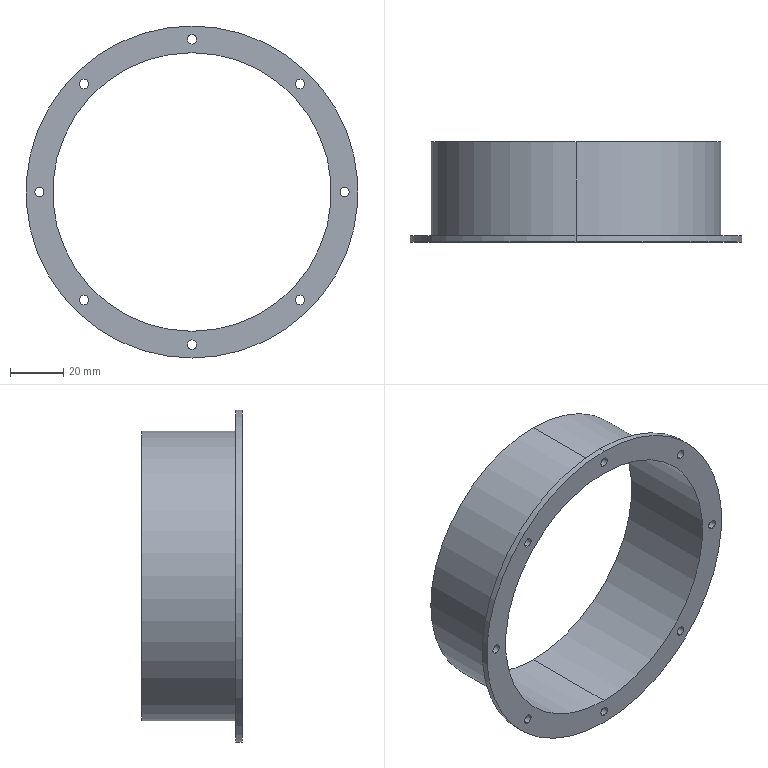Part | SolidWorks | features SavedExtBody 1 | 1 solid | 25 faces | box 124.775 x 37.645 x 124.775 mm | volume 33353 mm3 | cylinder 22 | plane 3 | commonest cylinder face diameters 3.5 x16 104.686 x2 108.906 x2 124.775 x2
STEP:
#1=CARTESIAN_POINT('',(-57.365,-225.737,66.75));
#2=VERTEX_POINT('',#1);
#3=CARTESIAN_POINT('',(-57.365,-225.737,63.25));
#4=VERTEX_POINT('',#3);
#5=CARTESIAN_POINT('',(-57.365,-225.737,65.));
#6=DIRECTION('',(0.,-1.,0.));
#7=DIRECTION('',(0.,0.,-1.));
#8=AXIS2_PLACEMENT_3D('',#5,#6,#7);
#9=CIRCLE('',#8,1.75);
#10=EDGE_CURVE('',#2,#4,#9,.T.);
#11=ORIENTED_EDGE('',*,*,#10,.F.);
#12=CARTESIAN_POINT('',(-57.365,-228.101,66.75));
#13=VERTEX_POINT('',#12);
#14=CARTESIAN_POINT('',(-57.365,-221.101,66.75));
#15=DIRECTION('',(0.,-1.,0.));
#16=VECTOR('',#15,1000.);
#17=LINE('',#14,#16);
#18=EDGE_CURVE('',#2,#13,#17,.T.);
#19=ORIENTED_EDGE('',*,*,#18,.T.);
#20=CARTESIAN_POINT('',(-57.365,-228.101,63.25));
#21=VERTEX_POINT('',#20);
#22=CARTESIAN_POINT('',(-57.365,-228.101,65.));
#23=DIRECTION('',(0.,-1.,0.));
#24=DIRECTION('',(0.,0.,-1.));
#25=AXIS2_PLACEMENT_3D('',#22,#23,#24);
#26=CIRCLE('',#25,1.75);
#27=EDGE_CURVE('',#13,#21,#26,.T.);
#28=ORIENTED_EDGE('',*,*,#27,.T.);
#29=CARTESIAN_POINT('',(-57.365,-221.101,63.25));
#30=DIRECTION('',(0.,-1.,0.));
#31=VECTOR('',#30,1000.);
#32=LINE('',#29,#31);
#33=EDGE_CURVE('',#4,#21,#32,.T.);
#34=ORIENTED_EDGE('',*,*,#33,.F.);
#35=EDGE_LOOP('',(#11,#19,#28,#34));
#36=FACE_OUTER_BOUND('',#35,.T.);
#37=CARTESIAN_POINT('',(-57.365,-221.101,65.));
#38=DIRECTION('',(0.,-1.,0.));
#39=DIRECTION('',(0.,0.,-1.));
#40=AXIS2_PLACEMENT_3D('',#37,#38,#39);
#41=CYLINDRICAL_SURFACE('',#40,1.75);
#42=ADVANCED_FACE('',(#36),#41,.F.);
#43=CARTESIAN_POINT('',(-40.563,-225.737,107.313));
#44=VERTEX_POINT('',#43);
#45=CARTESIAN_POINT('',(-40.563,-225.737,103.813));
#46=VERTEX_POINT('',#45);
#47=CARTESIAN_POINT('',(-40.563,-225.737,105.563));
#48=DIRECTION('',(0.,-1.,0.));
#49=DIRECTION('',(0.,0.,-1.));
#50=AXIS2_PLACEMENT_3D('',#47,#48,#49);
#51=CIRCLE('',#50,1.75);
#52=EDGE_CURVE('',#44,#46,#51,.T.);
#53=ORIENTED_EDGE('',*,*,#52,.F.);
#54=CARTESIAN_POINT('',(-40.563,-228.101,107.313));
#55=VERTEX_POINT('',#54);
#56=CARTESIAN_POINT('',(-40.563,-221.101,107.313));
#57=DIRECTION('',(0.,-1.,0.));
#58=VECTOR('',#57,1000.);
#59=LINE('',#56,#58);
#60=EDGE_CURVE('',#44,#55,#59,.T.);
#61=ORIENTED_EDGE('',*,*,#60,.T.);
#62=CARTESIAN_POINT('',(-40.563,-228.101,103.813));
#63=VERTEX_POINT('',#62);
#64=CARTESIAN_POINT('',(-40.563,-228.101,105.563));
#65=DIRECTION('',(0.,-1.,0.));
#66=DIRECTION('',(0.,0.,-1.));
#67=AXIS2_PLACEMENT_3D('',#64,#65,#66);
#68=CIRCLE('',#67,1.75);
#69=EDGE_CURVE('',#55,#63,#68,.T.);
#70=ORIENTED_EDGE('',*,*,#69,.T.);
#71=CARTESIAN_POINT('',(-40.563,-221.101,103.813));
#72=DIRECTION('',(0.,-1.,0.));
#73=VECTOR('',#72,1000.);
#74=LINE('',#71,#73);
#75=EDGE_CURVE('',#46,#63,#74,.T.);
#76=ORIENTED_EDGE('',*,*,#75,.F.);
#77=EDGE_LOOP('',(#53,#61,#70,#76));
#78=FACE_OUTER_BOUND('',#77,.T.);
#79=CARTESIAN_POINT('',(-40.563,-221.101,105.563));
#80=DIRECTION('',(0.,-1.,0.));
#81=DIRECTION('',(0.,0.,-1.));
#82=AXIS2_PLACEMENT_3D('',#79,#80,#81);
#83=CYLINDRICAL_SURFACE('',#82,1.75);
#84=ADVANCED_FACE('',(#78),#83,.F.);
#85=CARTESIAN_POINT('',(0.,-225.737,124.115));
#86=VERTEX_POINT('',#85);
#87=CARTESIAN_POINT('',(0.,-225.737,120.615));
#88=VERTEX_POINT('',#87);
#89=CARTESIAN_POINT('',(0.,-225.737,122.365));
#90=DIRECTION('',(0.,-1.,0.));
#91=DIRECTION('',(0.,0.,-1.));
#92=AXIS2_PLACEMENT_3D('',#89,#90,#91);
#93=CIRCLE('',#92,1.75);
#94=EDGE_CURVE('',#86,#88,#93,.T.);
#95=ORIENTED_EDGE('',*,*,#94,.F.);
#96=CARTESIAN_POINT('',(0.,-228.101,124.115));
#97=VERTEX_POINT('',#96);
#98=CARTESIAN_POINT('',(0.,-221.101,124.115));
#99=DIRECTION('',(0.,-1.,0.));
#100=VECTOR('',#99,1000.);
#101=LINE('',#98,#100);
#102=EDGE_CURVE('',#86,#97,#101,.T.);
#103=ORIENTED_EDGE('',*,*,#102,.T.);
#104=CARTESIAN_POINT('',(0.,-228.101,120.615));
#105=VERTEX_POINT('',#104);
#106=CARTESIAN_POINT('',(0.,-228.101,122.365));
#107=DIRECTION('',(0.,-1.,0.));
#108=DIRECTION('',(0.,0.,-1.));
#109=AXIS2_PLACEMENT_3D('',#106,#107,#108);
#110=CIRCLE('',#109,1.75);
#111=EDGE_CURVE('',#97,#105,#110,.T.);
#112=ORIENTED_EDGE('',*,*,#111,.T.);
#113=CARTESIAN_POINT('',(0.,-221.101,120.615));
#114=DIRECTION('',(0.,-1.,0.));
#115=VECTOR('',#114,1000.);
#116=LINE('',#113,#115);
#117=EDGE_CURVE('',#88,#105,#116,.T.);
#118=ORIENTED_EDGE('',*,*,#117,.F.);
#119=EDGE_LOOP('',(#95,#103,#112,#118));
#120=FACE_OUTER_BOUND('',#119,.T.);
#121=CARTESIAN_POINT('',(0.,-221.101,122.365));
#122=DIRECTION('',(0.,-1.,0.));
#123=DIRECTION('',(0.,0.,-1.));
#124=AXIS2_PLACEMENT_3D('',#121,#122,#123);
#125=CYLINDRICAL_SURFACE('',#124,1.75);
#126=ADVANCED_FACE('',(#120),#125,.F.);
#127=CARTESIAN_POINT('',(40.563,-225.737,107.313));
#128=VERTEX_POINT('',#127);
#129=CARTESIAN_POINT('',(40.563,-225.737,103.813));
#130=VERTEX_POINT('',#129);
#131=CARTESIAN_POINT('',(40.563,-225.737,105.563));
#132=DIRECTION('',(0.,-1.,0.));
#133=DIRECTION('',(0.,0.,-1.));
#134=AXIS2_PLACEMENT_3D('',#131,#132,#133);
#135=CIRCLE('',#134,1.75);
#136=EDGE_CURVE('',#128,#130,#135,.T.);
#137=ORIENTED_EDGE('',*,*,#136,.F.);
#138=CARTESIAN_POINT('',(40.563,-228.101,107.313));
#139=VERTEX_POINT('',#138);
#140=CARTESIAN_POINT('',(40.563,-221.101,107.313));
#141=DIRECTION('',(0.,-1.,0.));
#142=VECTOR('',#141,1000.);
#143=LINE('',#140,#142);
#144=EDGE_CURVE('',#128,#139,#143,.T.);
#145=ORIENTED_EDGE('',*,*,#144,.T.);
#146=CARTESIAN_POINT('',(40.563,-228.101,103.813));
#147=VERTEX_POINT('',#146);
#148=CARTESIAN_POINT('',(40.563,-228.101,105.563));
#149=DIRECTION('',(0.,-1.,0.));
#150=DIRECTION('',(0.,0.,-1.));
#151=AXIS2_PLACEMENT_3D('',#148,#149,#150);
#152=CIRCLE('',#151,1.75);
#153=EDGE_CURVE('',#139,#147,#152,.T.);
#154=ORIENTED_EDGE('',*,*,#153,.T.);
#155=CARTESIAN_POINT('',(40.563,-221.101,103.813));
#156=DIRECTION('',(0.,-1.,0.));
#157=VECTOR('',#156,1000.);
#158=LINE('',#155,#157);
#159=EDGE_CURVE('',#130,#147,#158,.T.);
#160=ORIENTED_EDGE('',*,*,#159,.F.);
#161=EDGE_LOOP('',(#137,#145,#154,#160));
#162=FACE_OUTER_BOUND('',#161,.T.);
#163=CARTESIAN_POINT('',(40.563,-221.101,105.563));
#164=DIRECTION('',(0.,-1.,0.));
#165=DIRECTION('',(0.,0.,-1.));
#166=AXIS2_PLACEMENT_3D('',#163,#164,#165);
#167=CYLINDRICAL_SURFACE('',#166,1.75);
#168=ADVANCED_FACE('',(#162),#167,.F.);
#169=CARTESIAN_POINT('',(57.365,-225.737,66.75));
#170=VERTEX_POINT('',#169);
#171=CARTESIAN_POINT('',(57.365,-225.737,63.25));
#172=VERTEX_POINT('',#171);
#173=CARTESIAN_POINT('',(57.365,-225.737,65.));
#174=DIRECTION('',(0.,-1.,0.));
#175=DIRECTION('',(0.,0.,-1.));
#176=AXIS2_PLACEMENT_3D('',#173,#174,#175);
#177=CIRCLE('',#176,1.75);
#178=EDGE_CURVE('',#170,#172,#177,.T.);
#179=ORIENTED_EDGE('',*,*,#178,.F.);
#180=CARTESIAN_POINT('',(57.365,-228.101,66.75));
#181=VERTEX_POINT('',#180);
#182=CARTESIAN_POINT('',(57.365,-221.101,66.75));
#183=DIRECTION('',(0.,-1.,0.));
#184=VECTOR('',#183,1000.);
#185=LINE('',#182,#184);
#186=EDGE_CURVE('',#170,#181,#185,.T.);
#187=ORIENTED_EDGE('',*,*,#186,.T.);
#188=CARTESIAN_POINT('',(57.365,-228.101,63.25));
#189=VERTEX_POINT('',#188);
#190=CARTESIAN_POINT('',(57.365,-228.101,65.));
#191=DIRECTION('',(0.,-1.,0.));
#192=DIRECTION('',(0.,0.,-1.));
#193=AXIS2_PLACEMENT_3D('',#190,#191,#192);
#194=CIRCLE('',#193,1.75);
#195=EDGE_CURVE('',#181,#189,#194,.T.);
#196=ORIENTED_EDGE('',*,*,#195,.T.);
#197=CARTESIAN_POINT('',(57.365,-221.101,63.25));
#198=DIRECTION('',(0.,-1.,0.));
#199=VECTOR('',#198,1000.);
#200=LINE('',#197,#199);
#201=EDGE_CURVE('',#172,#189,#200,.T.);
#202=ORIENTED_EDGE('',*,*,#201,.F.);
#203=EDGE_LOOP('',(#179,#187,#196,#202));
#204=FACE_OUTER_BOUND('',#203,.T.);
#205=CARTESIAN_POINT('',(57.365,-221.101,65.));
#206=DIRECTION('',(0.,-1.,0.));
#207=DIRECTION('',(0.,0.,-1.));
#208=AXIS2_PLACEMENT_3D('',#205,#206,#207);
#209=CYLINDRICAL_SURFACE('',#208,1.75);
#210=ADVANCED_FACE('',(#204),#209,.F.);
#211=CARTESIAN_POINT('',(40.563,-225.737,26.187));
#212=VERTEX_POINT('',#211);
#213=CARTESIAN_POINT('',(40.563,-225.737,22.687));
#214=VERTEX_POINT('',#213);
#215=CARTESIAN_POINT('',(40.563,-225.737,24.437));
#216=DIRECTION('',(0.,-1.,0.));
#217=DIRECTION('',(0.,0.,-1.));
#218=AXIS2_PLACEMENT_3D('',#215,#216,#217);
#219=CIRCLE('',#218,1.75);
#220=EDGE_CURVE('',#212,#214,#219,.T.);
#221=ORIENTED_EDGE('',*,*,#220,.F.);
#222=CARTESIAN_POINT('',(40.563,-228.101,26.187));
#223=VERTEX_POINT('',#222);
#224=CARTESIAN_POINT('',(40.563,-221.101,26.187));
#225=DIRECTION('',(0.,-1.,0.));
#226=VECTOR('',#225,1000.);
#227=LINE('',#224,#226);
#228=EDGE_CURVE('',#212,#223,#227,.T.);
#229=ORIENTED_EDGE('',*,*,#228,.T.);
#230=CARTESIAN_POINT('',(40.563,-228.101,22.687));
#231=VERTEX_POINT('',#230);
#232=CARTESIAN_POINT('',(40.563,-228.101,24.437));
#233=DIRECTION('',(0.,-1.,0.));
#234=DIRECTION('',(0.,0.,-1.));
#235=AXIS2_PLACEMENT_3D('',#232,#233,#234);
#236=CIRCLE('',#235,1.75);
#237=EDGE_CURVE('',#223,#231,#236,.T.);
#238=ORIENTED_EDGE('',*,*,#237,.T.);
#239=CARTESIAN_POINT('',(40.563,-221.101,22.687));
#240=DIRECTION('',(0.,-1.,0.));
#241=VECTOR('',#240,1000.);
#242=LINE('',#239,#241);
#243=EDGE_CURVE('',#214,#231,#242,.T.);
#244=ORIENTED_EDGE('',*,*,#243,.F.);
#245=EDGE_LOOP('',(#221,#229,#238,#244));
#246=FACE_OUTER_BOUND('',#245,.T.);
#247=CARTESIAN_POINT('',(40.563,-221.101,24.437));
#248=DIRECTION('',(0.,-1.,0.));
#249=DIRECTION('',(0.,0.,-1.));
#250=AXIS2_PLACEMENT_3D('',#247,#248,#249);
#251=CYLINDRICAL_SURFACE('',#250,1.75);
#252=ADVANCED_FACE('',(#246),#251,.F.);
#253=CARTESIAN_POINT('',(0.,-225.737,9.385));
#254=VERTEX_POINT('',#253);
#255=CARTESIAN_POINT('',(0.,-225.737,5.885));
#256=VERTEX_POINT('',#255);
#257=CARTESIAN_POINT('',(0.,-225.737,7.635));
#258=DIRECTION('',(0.,-1.,0.));
#259=DIRECTION('',(0.,0.,-1.));
#260=AXIS2_PLACEMENT_3D('',#257,#258,#259);
#261=CIRCLE('',#260,1.75);
#262=EDGE_CURVE('',#254,#256,#261,.T.);
#263=ORIENTED_EDGE('',*,*,#262,.F.);
#264=CARTESIAN_POINT('',(0.,-228.101,9.385));
#265=VERTEX_POINT('',#264);
#266=CARTESIAN_POINT('',(0.,-221.101,9.385));
#267=DIRECTION('',(0.,-1.,0.));
#268=VECTOR('',#267,1000.);
#269=LINE('',#266,#268);
#270=EDGE_CURVE('',#254,#265,#269,.T.);
#271=ORIENTED_EDGE('',*,*,#270,.T.);
#272=CARTESIAN_POINT('',(0.,-228.101,5.885));
#273=VERTEX_POINT('',#272);
#274=CARTESIAN_POINT('',(0.,-228.101,7.635));
#275=DIRECTION('',(0.,-1.,0.));
#276=DIRECTION('',(0.,0.,-1.));
#277=AXIS2_PLACEMENT_3D('',#274,#275,#276);
#278=CIRCLE('',#277,1.75);
#279=EDGE_CURVE('',#265,#273,#278,.T.);
#280=ORIENTED_EDGE('',*,*,#279,.T.);
#281=CARTESIAN_POINT('',(0.,-221.101,5.885));
#282=DIRECTION('',(0.,-1.,0.));
#283=VECTOR('',#282,1000.);
#284=LINE('',#281,#283);
#285=EDGE_CURVE('',#256,#273,#284,.T.);
#286=ORIENTED_EDGE('',*,*,#285,.F.);
#287=EDGE_LOOP('',(#263,#271,#280,#286));
#288=FACE_OUTER_BOUND('',#287,.T.);
#289=CARTESIAN_POINT('',(0.,-221.101,7.635));
#290=DIRECTION('',(0.,-1.,0.));
#291=DIRECTION('',(0.,0.,-1.));
#292=AXIS2_PLACEMENT_3D('',#289,#290,#291);
#293=CYLINDRICAL_SURFACE('',#292,1.75);
#294=ADVANCED_FACE('',(#288),#293,.F.);
#295=CARTESIAN_POINT('',(-40.563,-225.737,26.187));
#296=VERTEX_POINT('',#295);
#297=CARTESIAN_POINT('',(-40.563,-225.737,22.687));
#298=VERTEX_POINT('',#297);
#299=CARTESIAN_POINT('',(-40.563,-225.737,24.437));
#300=DIRECTION('',(0.,-1.,0.));
#301=DIRECTION('',(0.,0.,-1.));
#302=AXIS2_PLACEMENT_3D('',#299,#300,#301);
#303=CIRCLE('',#302,1.75);
#304=EDGE_CURVE('',#296,#298,#303,.T.);
#305=ORIENTED_EDGE('',*,*,#304,.F.);
#306=CARTESIAN_POINT('',(-40.563,-228.101,26.187));
#307=VERTEX_POINT('',#306);
#308=CARTESIAN_POINT('',(-40.563,-221.101,26.187));
#309=DIRECTION('',(0.,-1.,0.));
#310=VECTOR('',#309,1000.);
#311=LINE('',#308,#310);
#312=EDGE_CURVE('',#296,#307,#311,.T.);
#313=ORIENTED_EDGE('',*,*,#312,.T.);
#314=CARTESIAN_POINT('',(-40.563,-228.101,22.687));
#315=VERTEX_POINT('',#314);
#316=CARTESIAN_POINT('',(-40.563,-228.101,24.437));
#317=DIRECTION('',(0.,-1.,0.));
#318=DIRECTION('',(0.,0.,-1.));
#319=AXIS2_PLACEMENT_3D('',#316,#317,#318);
#320=CIRCLE('',#319,1.75);
#321=EDGE_CURVE('',#307,#315,#320,.T.);
#322=ORIENTED_EDGE('',*,*,#321,.T.);
#323=CARTESIAN_POINT('',(-40.563,-221.101,22.687));
#324=DIRECTION('',(0.,-1.,0.));
#325=VECTOR('',#324,1000.);
#326=LINE('',#323,#325);
#327=EDGE_CURVE('',#298,#315,#326,.T.);
#328=ORIENTED_EDGE('',*,*,#327,.F.);
#329=EDGE_LOOP('',(#305,#313,#322,#328));
#330=FACE_OUTER_BOUND('',#329,.T.);
#331=CARTESIAN_POINT('',(-40.563,-221.101,24.437));
#332=DIRECTION('',(0.,-1.,0.));
#333=DIRECTION('',(0.,0.,-1.));
#334=AXIS2_PLACEMENT_3D('',#331,#332,#333);
#335=CYLINDRICAL_SURFACE('',#334,1.75);
#336=ADVANCED_FACE('',(#330),#335,.F.);
#337=CARTESIAN_POINT('',(0.,-190.456,10.547));
#338=VERTEX_POINT('',#337);
#339=CARTESIAN_POINT('',(0.,-190.456,119.453));
#340=VERTEX_POINT('',#339);
#341=CARTESIAN_POINT('',(0.,-190.456,65.));
#342=DIRECTION('',(0.,-1.,0.));
#343=DIRECTION('',(0.,0.,-1.));
#344=AXIS2_PLACEMENT_3D('',#341,#342,#343);
#345=CIRCLE('',#344,54.453);
#346=EDGE_CURVE('',#338,#340,#345,.T.);
#347=ORIENTED_EDGE('',*,*,#346,.T.);
#348=CARTESIAN_POINT('',(0.,-225.737,119.453));
#349=VERTEX_POINT('',#348);
#350=CARTESIAN_POINT('',(0.,-253.035,119.453));
#351=DIRECTION('',(0.,-1.,0.));
#352=VECTOR('',#351,1000.);
#353=LINE('',#350,#352);
#354=EDGE_CURVE('',#340,#349,#353,.T.);
#355=ORIENTED_EDGE('',*,*,#354,.T.);
#356=CARTESIAN_POINT('',(0.,-225.737,10.547));
#357=VERTEX_POINT('',#356);
#358=CARTESIAN_POINT('',(0.,-225.737,65.));
#359=DIRECTION('',(0.,-1.,0.));
#360=DIRECTION('',(0.,0.,-1.));
#361=AXIS2_PLACEMENT_3D('',#358,#359,#360);
#362=CIRCLE('',#361,54.453);
#363=EDGE_CURVE('',#357,#349,#362,.T.);
#364=ORIENTED_EDGE('',*,*,#363,.F.);
#365=CARTESIAN_POINT('',(0.,-253.035,10.547));
#366=DIRECTION('',(0.,-1.,0.));
#367=VECTOR('',#366,1000.);
#368=LINE('',#365,#367);
#369=EDGE_CURVE('',#338,#357,#368,.T.);
#370=ORIENTED_EDGE('',*,*,#369,.F.);
#371=EDGE_LOOP('',(#347,#355,#364,#370));
#372=FACE_OUTER_BOUND('',#371,.T.);
#373=CARTESIAN_POINT('',(0.,-253.035,65.));
#374=DIRECTION('',(0.,-1.,0.));
#375=DIRECTION('',(0.,0.,-1.));
#376=AXIS2_PLACEMENT_3D('',#373,#374,#375);
#377=CYLINDRICAL_SURFACE('',#376,54.453);
#378=ADVANCED_FACE('',(#372),#377,.T.);
#379=CARTESIAN_POINT('',(0.,-225.737,2.613));
#380=VERTEX_POINT('',#379);
#381=CARTESIAN_POINT('',(0.,-225.737,127.387));
#382=VERTEX_POINT('',#381);
#383=CARTESIAN_POINT('',(0.,-225.737,65.));
#384=DIRECTION('',(0.,-1.,0.));
#385=DIRECTION('',(0.,0.,-1.));
#386=AXIS2_PLACEMENT_3D('',#383,#384,#385);
#387=CIRCLE('',#386,62.387);
#388=EDGE_CURVE('',#380,#382,#387,.T.);
#389=ORIENTED_EDGE('',*,*,#388,.T.);
#390=CARTESIAN_POINT('',(0.,-228.101,127.387));
#391=VERTEX_POINT('',#390);
#392=CARTESIAN_POINT('',(0.,-253.035,127.387));
#393=DIRECTION('',(0.,-1.,0.));
#394=VECTOR('',#393,1000.);
#395=LINE('',#392,#394);
#396=EDGE_CURVE('',#382,#391,#395,.T.);
#397=ORIENTED_EDGE('',*,*,#396,.T.);
#398=CARTESIAN_POINT('',(0.,-228.101,2.613));
#399=VERTEX_POINT('',#398);
#400=CARTESIAN_POINT('',(0.,-228.101,65.));
#401=DIRECTION('',(0.,-1.,0.));
#402=DIRECTION('',(0.,0.,-1.));
#403=AXIS2_PLACEMENT_3D('',#400,#401,#402);
#404=CIRCLE('',#403,62.387);
#405=EDGE_CURVE('',#399,#391,#404,.T.);
#406=ORIENTED_EDGE('',*,*,#405,.F.);
#407=CARTESIAN_POINT('',(0.,-253.035,2.613));
#408=DIRECTION('',(0.,-1.,0.));
#409=VECTOR('',#408,1000.);
#410=LINE('',#407,#409);
#411=EDGE_CURVE('',#380,#399,#410,.T.);
#412=ORIENTED_EDGE('',*,*,#411,.F.);
#413=EDGE_LOOP('',(#389,#397,#406,#412));
#414=FACE_OUTER_BOUND('',#413,.T.);
#415=CARTESIAN_POINT('',(0.,-253.035,65.));
#416=DIRECTION('',(0.,-1.,0.));
#417=DIRECTION('',(0.,0.,-1.));
#418=AXIS2_PLACEMENT_3D('',#415,#416,#417);
#419=CYLINDRICAL_SURFACE('',#418,62.387);
#420=ADVANCED_FACE('',(#414),#419,.T.);
#421=CARTESIAN_POINT('',(0.,-190.456,117.343));
#422=VERTEX_POINT('',#421);
#423=CARTESIAN_POINT('',(0.,-190.456,12.657));
#424=VERTEX_POINT('',#423);
#425=CARTESIAN_POINT('',(0.,-190.456,65.));
#426=DIRECTION('',(0.,-1.,0.));
#427=DIRECTION('',(0.,0.,-1.));
#428=AXIS2_PLACEMENT_3D('',#425,#426,#427);
#429=CIRCLE('',#428,52.343);
#430=EDGE_CURVE('',#422,#424,#429,.T.);
#431=ORIENTED_EDGE('',*,*,#430,.F.);
#432=CARTESIAN_POINT('',(0.,-228.101,117.343));
#433=VERTEX_POINT('',#432);
#434=CARTESIAN_POINT('',(0.,-253.035,117.343));
#435=DIRECTION('',(0.,-1.,0.));
#436=VECTOR('',#435,1000.);
#437=LINE('',#434,#436);
#438=EDGE_CURVE('',#422,#433,#437,.T.);
#439=ORIENTED_EDGE('',*,*,#438,.T.);
#440=CARTESIAN_POINT('',(0.,-228.101,12.657));
#441=VERTEX_POINT('',#440);
#442=CARTESIAN_POINT('',(0.,-228.101,65.));
#443=DIRECTION('',(0.,-1.,0.));
#444=DIRECTION('',(0.,0.,-1.));
#445=AXIS2_PLACEMENT_3D('',#442,#443,#444);
#446=CIRCLE('',#445,52.343);
#447=EDGE_CURVE('',#433,#441,#446,.T.);
#448=ORIENTED_EDGE('',*,*,#447,.T.);
#449=CARTESIAN_POINT('',(0.,-253.035,12.657));
#450=DIRECTION('',(0.,-1.,0.));
#451=VECTOR('',#450,1000.);
#452=LINE('',#449,#451);
#453=EDGE_CURVE('',#424,#441,#452,.T.);
#454=ORIENTED_EDGE('',*,*,#453,.F.);
#455=EDGE_LOOP('',(#431,#439,#448,#454));
#456=FACE_OUTER_BOUND('',#455,.T.);
#457=CARTESIAN_POINT('',(0.,-253.035,65.));
#458=DIRECTION('',(0.,-1.,0.));
#459=DIRECTION('',(0.,0.,-1.));
#460=AXIS2_PLACEMENT_3D('',#457,#458,#459);
#461=CYLINDRICAL_SURFACE('',#460,52.343);
#462=ADVANCED_FACE('',(#456),#461,.F.);
#463=ORIENTED_EDGE('',*,*,#438,.F.);
#464=CARTESIAN_POINT('',(0.,-190.456,65.));
#465=DIRECTION('',(0.,-1.,0.));
#466=DIRECTION('',(0.,0.,-1.));
#467=AXIS2_PLACEMENT_3D('',#464,#465,#466);
#468=CIRCLE('',#467,52.343);
#469=EDGE_CURVE('',#424,#422,#468,.T.);
#470=ORIENTED_EDGE('',*,*,#469,.F.);
#471=ORIENTED_EDGE('',*,*,#453,.T.);
#472=CARTESIAN_POINT('',(0.,-228.101,65.));
#473=DIRECTION('',(0.,-1.,0.));
#474=DIRECTION('',(0.,0.,-1.));
#475=AXIS2_PLACEMENT_3D('',#472,#473,#474);
#476=CIRCLE('',#475,52.343);
#477=EDGE_CURVE('',#441,#433,#476,.T.);
#478=ORIENTED_EDGE('',*,*,#477,.T.);
#479=EDGE_LOOP('',(#463,#470,#471,#478));
#480=FACE_OUTER_BOUND('',#479,.T.);
#481=CARTESIAN_POINT('',(0.,-253.035,65.));
#482=DIRECTION('',(0.,-1.,0.));
#483=DIRECTION('',(0.,0.,-1.));
#484=AXIS2_PLACEMENT_3D('',#481,#482,#483);
#485=CYLINDRICAL_SURFACE('',#484,52.343);
#486=ADVANCED_FACE('',(#480),#485,.F.);
#487=CARTESIAN_POINT('',(-57.365,-228.101,65.));
#488=DIRECTION('',(0.,-1.,0.));
#489=DIRECTION('',(0.,0.,-1.));
#490=AXIS2_PLACEMENT_3D('',#487,#488,#489);
#491=CIRCLE('',#490,1.75);
#492=EDGE_CURVE('',#21,#13,#491,.T.);
#493=ORIENTED_EDGE('',*,*,#492,.F.);
#494=ORIENTED_EDGE('',*,*,#27,.F.);
#495=EDGE_LOOP('',(#493,#494));
#496=FACE_BOUND('',#495,.T.);
#497=CARTESIAN_POINT('',(-40.563,-228.101,105.563));
#498=DIRECTION('',(0.,-1.,0.));
#499=DIRECTION('',(0.,0.,-1.));
#500=AXIS2_PLACEMENT_3D('',#497,#498,#499);
#501=CIRCLE('',#500,1.75);
#502=EDGE_CURVE('',#63,#55,#501,.T.);
#503=ORIENTED_EDGE('',*,*,#502,.F.);
#504=ORIENTED_EDGE('',*,*,#69,.F.);
#505=EDGE_LOOP('',(#503,#504));
#506=FACE_BOUND('',#505,.T.);
#507=CARTESIAN_POINT('',(0.,-228.101,122.365));
#508=DIRECTION('',(0.,-1.,0.));
#509=DIRECTION('',(0.,0.,-1.));
#510=AXIS2_PLACEMENT_3D('',#507,#508,#509);
#511=CIRCLE('',#510,1.75);
#512=EDGE_CURVE('',#105,#97,#511,.T.);
#513=ORIENTED_EDGE('',*,*,#512,.F.);
#514=ORIENTED_EDGE('',*,*,#111,.F.);
#515=EDGE_LOOP('',(#513,#514));
#516=FACE_BOUND('',#515,.T.);
#517=CARTESIAN_POINT('',(40.563,-228.101,105.563));
#518=DIRECTION('',(0.,-1.,0.));
#519=DIRECTION('',(0.,0.,-1.));
#520=AXIS2_PLACEMENT_3D('',#517,#518,#519);
#521=CIRCLE('',#520,1.75);
#522=EDGE_CURVE('',#147,#139,#521,.T.);
#523=ORIENTED_EDGE('',*,*,#522,.F.);
#524=ORIENTED_EDGE('',*,*,#153,.F.);
#525=EDGE_LOOP('',(#523,#524));
#526=FACE_BOUND('',#525,.T.);
#527=CARTESIAN_POINT('',(57.365,-228.101,65.));
#528=DIRECTION('',(0.,-1.,0.));
#529=DIRECTION('',(0.,0.,-1.));
#530=AXIS2_PLACEMENT_3D('',#527,#528,#529);
#531=CIRCLE('',#530,1.75);
#532=EDGE_CURVE('',#189,#181,#531,.T.);
#533=ORIENTED_EDGE('',*,*,#532,.F.);
#534=ORIENTED_EDGE('',*,*,#195,.F.);
#535=EDGE_LOOP('',(#533,#534));
#536=FACE_BOUND('',#535,.T.);
#537=CARTESIAN_POINT('',(40.563,-228.101,24.437));
#538=DIRECTION('',(0.,-1.,0.));
#539=DIRECTION('',(0.,0.,-1.));
#540=AXIS2_PLACEMENT_3D('',#537,#538,#539);
#541=CIRCLE('',#540,1.75);
#542=EDGE_CURVE('',#231,#223,#541,.T.);
#543=ORIENTED_EDGE('',*,*,#542,.F.);
#544=ORIENTED_EDGE('',*,*,#237,.F.);
#545=EDGE_LOOP('',(#543,#544));
#546=FACE_BOUND('',#545,.T.);
#547=CARTESIAN_POINT('',(0.,-228.101,7.635));
#548=DIRECTION('',(0.,-1.,0.));
#549=DIRECTION('',(0.,0.,-1.));
#550=AXIS2_PLACEMENT_3D('',#547,#548,#549);
#551=CIRCLE('',#550,1.75);
#552=EDGE_CURVE('',#273,#265,#551,.T.);
#553=ORIENTED_EDGE('',*,*,#552,.F.);
#554=ORIENTED_EDGE('',*,*,#279,.F.);
#555=EDGE_LOOP('',(#553,#554));
#556=FACE_BOUND('',#555,.T.);
#557=CARTESIAN_POINT('',(-40.563,-228.101,24.437));
#558=DIRECTION('',(0.,-1.,0.));
#559=DIRECTION('',(0.,0.,-1.));
#560=AXIS2_PLACEMENT_3D('',#557,#558,#559);
#561=CIRCLE('',#560,1.75);
#562=EDGE_CURVE('',#315,#307,#561,.T.);
#563=ORIENTED_EDGE('',*,*,#562,.F.);
#564=ORIENTED_EDGE('',*,*,#321,.F.);
#565=EDGE_LOOP('',(#563,#564));
#566=FACE_BOUND('',#565,.T.);
#567=ORIENTED_EDGE('',*,*,#477,.F.);
#568=ORIENTED_EDGE('',*,*,#447,.F.);
#569=EDGE_LOOP('',(#567,#568));
#570=FACE_BOUND('',#569,.T.);
#571=ORIENTED_EDGE('',*,*,#405,.T.);
#572=CARTESIAN_POINT('',(0.,-228.101,65.));
#573=DIRECTION('',(0.,-1.,0.));
#574=DIRECTION('',(0.,0.,-1.));
#575=AXIS2_PLACEMENT_3D('',#572,#573,#574);
#576=CIRCLE('',#575,62.387);
#577=EDGE_CURVE('',#391,#399,#576,.T.);
#578=ORIENTED_EDGE('',*,*,#577,.T.);
#579=EDGE_LOOP('',(#571,#578));
#580=FACE_OUTER_BOUND('',#579,.T.);
#581=CARTESIAN_POINT('',(-54.453,-228.101,65.));
#582=DIRECTION('',(0.,1.,0.));
#583=DIRECTION('',(0.,0.,1.));
#584=AXIS2_PLACEMENT_3D('',#581,#582,#583);
#585=PLANE('',#584);
#586=ADVANCED_FACE('',(#496,#506,#516,#526,#536,#546,#556,#566,#570,#580),#585,.F.);
#587=ORIENTED_EDGE('',*,*,#396,.F.);
#588=CARTESIAN_POINT('',(0.,-225.737,65.));
#589=DIRECTION('',(0.,-1.,0.));
#590=DIRECTION('',(0.,0.,-1.));
#591=AXIS2_PLACEMENT_3D('',#588,#589,#590);
#592=CIRCLE('',#591,62.387);
#593=EDGE_CURVE('',#382,#380,#592,.T.);
#594=ORIENTED_EDGE('',*,*,#593,.T.);
#595=ORIENTED_EDGE('',*,*,#411,.T.);
#596=ORIENTED_EDGE('',*,*,#577,.F.);
#597=EDGE_LOOP('',(#587,#594,#595,#596));
#598=FACE_OUTER_BOUND('',#597,.T.);
#599=CARTESIAN_POINT('',(0.,-253.035,65.));
#600=DIRECTION('',(0.,-1.,0.));
#601=DIRECTION('',(0.,0.,-1.));
#602=AXIS2_PLACEMENT_3D('',#599,#600,#601);
#603=CYLINDRICAL_SURFACE('',#602,62.387);
#604=ADVANCED_FACE('',(#598),#603,.T.);
#605=CARTESIAN_POINT('',(-57.365,-225.737,65.));
#606=DIRECTION('',(0.,-1.,0.));
#607=DIRECTION('',(0.,0.,-1.));
#608=AXIS2_PLACEMENT_3D('',#605,#606,#607);
#609=CIRCLE('',#608,1.75);
#610=EDGE_CURVE('',#4,#2,#609,.T.);
#611=ORIENTED_EDGE('',*,*,#610,.T.);
#612=ORIENTED_EDGE('',*,*,#10,.T.);
#613=EDGE_LOOP('',(#611,#612));
#614=FACE_BOUND('',#613,.T.);
#615=CARTESIAN_POINT('',(-40.563,-225.737,105.563));
#616=DIRECTION('',(0.,-1.,0.));
#617=DIRECTION('',(0.,0.,-1.));
#618=AXIS2_PLACEMENT_3D('',#615,#616,#617);
#619=CIRCLE('',#618,1.75);
#620=EDGE_CURVE('',#46,#44,#619,.T.);
#621=ORIENTED_EDGE('',*,*,#620,.T.);
#622=ORIENTED_EDGE('',*,*,#52,.T.);
#623=EDGE_LOOP('',(#621,#622));
#624=FACE_BOUND('',#623,.T.);
#625=CARTESIAN_POINT('',(0.,-225.737,122.365));
#626=DIRECTION('',(0.,-1.,0.));
#627=DIRECTION('',(0.,0.,-1.));
#628=AXIS2_PLACEMENT_3D('',#625,#626,#627);
#629=CIRCLE('',#628,1.75);
#630=EDGE_CURVE('',#88,#86,#629,.T.);
#631=ORIENTED_EDGE('',*,*,#630,.T.);
#632=ORIENTED_EDGE('',*,*,#94,.T.);
#633=EDGE_LOOP('',(#631,#632));
#634=FACE_BOUND('',#633,.T.);
#635=CARTESIAN_POINT('',(40.563,-225.737,105.563));
#636=DIRECTION('',(0.,-1.,0.));
#637=DIRECTION('',(0.,0.,-1.));
#638=AXIS2_PLACEMENT_3D('',#635,#636,#637);
#639=CIRCLE('',#638,1.75);
#640=EDGE_CURVE('',#130,#128,#639,.T.);
#641=ORIENTED_EDGE('',*,*,#640,.T.);
#642=ORIENTED_EDGE('',*,*,#136,.T.);
#643=EDGE_LOOP('',(#641,#642));
#644=FACE_BOUND('',#643,.T.);
#645=CARTESIAN_POINT('',(57.365,-225.737,65.));
#646=DIRECTION('',(0.,-1.,0.));
#647=DIRECTION('',(0.,0.,-1.));
#648=AXIS2_PLACEMENT_3D('',#645,#646,#647);
#649=CIRCLE('',#648,1.75);
#650=EDGE_CURVE('',#172,#170,#649,.T.);
#651=ORIENTED_EDGE('',*,*,#650,.T.);
#652=ORIENTED_EDGE('',*,*,#178,.T.);
#653=EDGE_LOOP('',(#651,#652));
#654=FACE_BOUND('',#653,.T.);
#655=CARTESIAN_POINT('',(40.563,-225.737,24.437));
#656=DIRECTION('',(0.,-1.,0.));
#657=DIRECTION('',(0.,0.,-1.));
#658=AXIS2_PLACEMENT_3D('',#655,#656,#657);
#659=CIRCLE('',#658,1.75);
#660=EDGE_CURVE('',#214,#212,#659,.T.);
#661=ORIENTED_EDGE('',*,*,#660,.T.);
#662=ORIENTED_EDGE('',*,*,#220,.T.);
#663=EDGE_LOOP('',(#661,#662));
#664=FACE_BOUND('',#663,.T.);
#665=CARTESIAN_POINT('',(0.,-225.737,7.635));
#666=DIRECTION('',(0.,-1.,0.));
#667=DIRECTION('',(0.,0.,-1.));
#668=AXIS2_PLACEMENT_3D('',#665,#666,#667);
#669=CIRCLE('',#668,1.75);
#670=EDGE_CURVE('',#256,#254,#669,.T.);
#671=ORIENTED_EDGE('',*,*,#670,.T.);
#672=ORIENTED_EDGE('',*,*,#262,.T.);
#673=EDGE_LOOP('',(#671,#672));
#674=FACE_BOUND('',#673,.T.);
#675=CARTESIAN_POINT('',(-40.563,-225.737,24.437));
#676=DIRECTION('',(0.,-1.,0.));
#677=DIRECTION('',(0.,0.,-1.));
#678=AXIS2_PLACEMENT_3D('',#675,#676,#677);
#679=CIRCLE('',#678,1.75);
#680=EDGE_CURVE('',#298,#296,#679,.T.);
#681=ORIENTED_EDGE('',*,*,#680,.T.);
#682=ORIENTED_EDGE('',*,*,#304,.T.);
#683=EDGE_LOOP('',(#681,#682));
#684=FACE_BOUND('',#683,.T.);
#685=ORIENTED_EDGE('',*,*,#388,.F.);
#686=ORIENTED_EDGE('',*,*,#593,.F.);
#687=EDGE_LOOP('',(#685,#686));
#688=FACE_OUTER_BOUND('',#687,.T.);
#689=ORIENTED_EDGE('',*,*,#363,.T.);
#690=CARTESIAN_POINT('',(0.,-225.737,65.));
#691=DIRECTION('',(0.,-1.,0.));
#692=DIRECTION('',(0.,0.,-1.));
#693=AXIS2_PLACEMENT_3D('',#690,#691,#692);
#694=CIRCLE('',#693,54.453);
#695=EDGE_CURVE('',#349,#357,#694,.T.);
#696=ORIENTED_EDGE('',*,*,#695,.T.);
#697=EDGE_LOOP('',(#689,#696));
#698=FACE_BOUND('',#697,.T.);
#699=CARTESIAN_POINT('',(-54.453,-225.737,65.));
#700=DIRECTION('',(0.,-1.,0.));
#701=DIRECTION('',(0.,0.,-1.));
#702=AXIS2_PLACEMENT_3D('',#699,#700,#701);
#703=PLANE('',#702);
#704=ADVANCED_FACE('',(#614,#624,#634,#644,#654,#664,#674,#684,#688,#698),#703,.F.);
#705=ORIENTED_EDGE('',*,*,#354,.F.);
#706=CARTESIAN_POINT('',(0.,-190.456,65.));
#707=DIRECTION('',(0.,-1.,0.));
#708=DIRECTION('',(0.,0.,-1.));
#709=AXIS2_PLACEMENT_3D('',#706,#707,#708);
#710=CIRCLE('',#709,54.453);
#711=EDGE_CURVE('',#340,#338,#710,.T.);
#712=ORIENTED_EDGE('',*,*,#711,.T.);
#713=ORIENTED_EDGE('',*,*,#369,.T.);
#714=ORIENTED_EDGE('',*,*,#695,.F.);
#715=EDGE_LOOP('',(#705,#712,#713,#714));
#716=FACE_OUTER_BOUND('',#715,.T.);
#717=CARTESIAN_POINT('',(0.,-253.035,65.));
#718=DIRECTION('',(0.,-1.,0.));
#719=DIRECTION('',(0.,0.,-1.));
#720=AXIS2_PLACEMENT_3D('',#717,#718,#719);
#721=CYLINDRICAL_SURFACE('',#720,54.453);
#722=ADVANCED_FACE('',(#716),#721,.T.);
#723=ORIENTED_EDGE('',*,*,#346,.F.);
#724=ORIENTED_EDGE('',*,*,#711,.F.);
#725=EDGE_LOOP('',(#723,#724));
#726=FACE_OUTER_BOUND('',#725,.T.);
#727=ORIENTED_EDGE('',*,*,#469,.T.);
#728=ORIENTED_EDGE('',*,*,#430,.T.);
#729=EDGE_LOOP('',(#727,#728));
#730=FACE_BOUND('',#729,.T.);
#731=CARTESIAN_POINT('',(-52.343,-190.456,65.));
#732=DIRECTION('',(0.,-1.,0.));
#733=DIRECTION('',(0.,0.,-1.));
#734=AXIS2_PLACEMENT_3D('',#731,#732,#733);
#735=PLANE('',#734);
#736=ADVANCED_FACE('',(#726,#730),#735,.F.);
#737=ORIENTED_EDGE('',*,*,#312,.F.);
#738=ORIENTED_EDGE('',*,*,#680,.F.);
#739=ORIENTED_EDGE('',*,*,#327,.T.);
#740=ORIENTED_EDGE('',*,*,#562,.T.);
#741=EDGE_LOOP('',(#737,#738,#739,#740));
#742=FACE_OUTER_BOUND('',#741,.T.);
#743=CARTESIAN_POINT('',(-40.563,-221.101,24.437));
#744=DIRECTION('',(0.,-1.,0.));
#745=DIRECTION('',(0.,0.,-1.));
#746=AXIS2_PLACEMENT_3D('',#743,#744,#745);
#747=CYLINDRICAL_SURFACE('',#746,1.75);
#748=ADVANCED_FACE('',(#742),#747,.F.);
#749=ORIENTED_EDGE('',*,*,#270,.F.);
#750=ORIENTED_EDGE('',*,*,#670,.F.);
#751=ORIENTED_EDGE('',*,*,#285,.T.);
#752=ORIENTED_EDGE('',*,*,#552,.T.);
#753=EDGE_LOOP('',(#749,#750,#751,#752));
#754=FACE_OUTER_BOUND('',#753,.T.);
#755=CARTESIAN_POINT('',(0.,-221.101,7.635));
#756=DIRECTION('',(0.,-1.,0.));
#757=DIRECTION('',(0.,0.,-1.));
#758=AXIS2_PLACEMENT_3D('',#755,#756,#757);
#759=CYLINDRICAL_SURFACE('',#758,1.75);
#760=ADVANCED_FACE('',(#754),#759,.F.);
#761=ORIENTED_EDGE('',*,*,#228,.F.);
#762=ORIENTED_EDGE('',*,*,#660,.F.);
#763=ORIENTED_EDGE('',*,*,#243,.T.);
#764=ORIENTED_EDGE('',*,*,#542,.T.);
#765=EDGE_LOOP('',(#761,#762,#763,#764));
#766=FACE_OUTER_BOUND('',#765,.T.);
#767=CARTESIAN_POINT('',(40.563,-221.101,24.437));
#768=DIRECTION('',(0.,-1.,0.));
#769=DIRECTION('',(0.,0.,-1.));
#770=AXIS2_PLACEMENT_3D('',#767,#768,#769);
#771=CYLINDRICAL_SURFACE('',#770,1.75);
#772=ADVANCED_FACE('',(#766),#771,.F.);
#773=ORIENTED_EDGE('',*,*,#186,.F.);
#774=ORIENTED_EDGE('',*,*,#650,.F.);
#775=ORIENTED_EDGE('',*,*,#201,.T.);
#776=ORIENTED_EDGE('',*,*,#532,.T.);
#777=EDGE_LOOP('',(#773,#774,#775,#776));
#778=FACE_OUTER_BOUND('',#777,.T.);
#779=CARTESIAN_POINT('',(57.365,-221.101,65.));
#780=DIRECTION('',(0.,-1.,0.));
#781=DIRECTION('',(0.,0.,-1.));
#782=AXIS2_PLACEMENT_3D('',#779,#780,#781);
#783=CYLINDRICAL_SURFACE('',#782,1.75);
#784=ADVANCED_FACE('',(#778),#783,.F.);
#785=ORIENTED_EDGE('',*,*,#144,.F.);
#786=ORIENTED_EDGE('',*,*,#640,.F.);
#787=ORIENTED_EDGE('',*,*,#159,.T.);
#788=ORIENTED_EDGE('',*,*,#522,.T.);
#789=EDGE_LOOP('',(#785,#786,#787,#788));
#790=FACE_OUTER_BOUND('',#789,.T.);
#791=CARTESIAN_POINT('',(40.563,-221.101,105.563));
#792=DIRECTION('',(0.,-1.,0.));
#793=DIRECTION('',(0.,0.,-1.));
#794=AXIS2_PLACEMENT_3D('',#791,#792,#793);
#795=CYLINDRICAL_SURFACE('',#794,1.75);
#796=ADVANCED_FACE('',(#790),#795,.F.);
#797=ORIENTED_EDGE('',*,*,#102,.F.);
#798=ORIENTED_EDGE('',*,*,#630,.F.);
#799=ORIENTED_EDGE('',*,*,#117,.T.);
#800=ORIENTED_EDGE('',*,*,#512,.T.);
#801=EDGE_LOOP('',(#797,#798,#799,#800));
#802=FACE_OUTER_BOUND('',#801,.T.);
#803=CARTESIAN_POINT('',(0.,-221.101,122.365));
#804=DIRECTION('',(0.,-1.,0.));
#805=DIRECTION('',(0.,0.,-1.));
#806=AXIS2_PLACEMENT_3D('',#803,#804,#805);
#807=CYLINDRICAL_SURFACE('',#806,1.75);
#808=ADVANCED_FACE('',(#802),#807,.F.);
#809=ORIENTED_EDGE('',*,*,#60,.F.);
#810=ORIENTED_EDGE('',*,*,#620,.F.);
#811=ORIENTED_EDGE('',*,*,#75,.T.);
#812=ORIENTED_EDGE('',*,*,#502,.T.);
#813=EDGE_LOOP('',(#809,#810,#811,#812));
#814=FACE_OUTER_BOUND('',#813,.T.);
#815=CARTESIAN_POINT('',(-40.563,-221.101,105.563));
#816=DIRECTION('',(0.,-1.,0.));
#817=DIRECTION('',(0.,0.,-1.));
#818=AXIS2_PLACEMENT_3D('',#815,#816,#817);
#819=CYLINDRICAL_SURFACE('',#818,1.75);
#820=ADVANCED_FACE('',(#814),#819,.F.);
#821=ORIENTED_EDGE('',*,*,#18,.F.);
#822=ORIENTED_EDGE('',*,*,#610,.F.);
#823=ORIENTED_EDGE('',*,*,#33,.T.);
#824=ORIENTED_EDGE('',*,*,#492,.T.);
#825=EDGE_LOOP('',(#821,#822,#823,#824));
#826=FACE_OUTER_BOUND('',#825,.T.);
#827=CARTESIAN_POINT('',(-57.365,-221.101,65.));
#828=DIRECTION('',(0.,-1.,0.));
#829=DIRECTION('',(0.,0.,-1.));
#830=AXIS2_PLACEMENT_3D('',#827,#828,#829);
#831=CYLINDRICAL_SURFACE('',#830,1.75);
#832=ADVANCED_FACE('',(#826),#831,.F.);
#833=CLOSED_SHELL('',(#42,#84,#126,#168,#210,#252,#294,#336,#378,#420,#462,#486,#586,#604,#704,#722,#736,#748,#760,#772,#784,#796,#808,#820,#832));
#834=MANIFOLD_SOLID_BREP('',#833);
#835=CARTESIAN_POINT('',(0.,0.,0.));
#836=DIRECTION('',(0.,0.,1.));
#837=DIRECTION('',(1.,0.,0.));
#838=AXIS2_PLACEMENT_3D('',#835,#836,#837);
#839=(LENGTH_UNIT()NAMED_UNIT(*)SI_UNIT(.MILLI.,.METRE.));
#840=UNCERTAINTY_MEASURE_WITH_UNIT(LENGTH_MEASURE(0.00001),#839,'','');
#841=(NAMED_UNIT(*)PLANE_ANGLE_UNIT()SI_UNIT($,.RADIAN.));
#842=(NAMED_UNIT(*)SI_UNIT($,.STERADIAN.)SOLID_ANGLE_UNIT());
#843=(GEOMETRIC_REPRESENTATION_CONTEXT(3)GLOBAL_UNCERTAINTY_ASSIGNED_CONTEXT((#840))GLOBAL_UNIT_ASSIGNED_CONTEXT((#839,#841,#842))REPRESENTATION_CONTEXT('',''));
#844=ADVANCED_BREP_SHAPE_REPRESENTATION('',(#834,#838),#843);